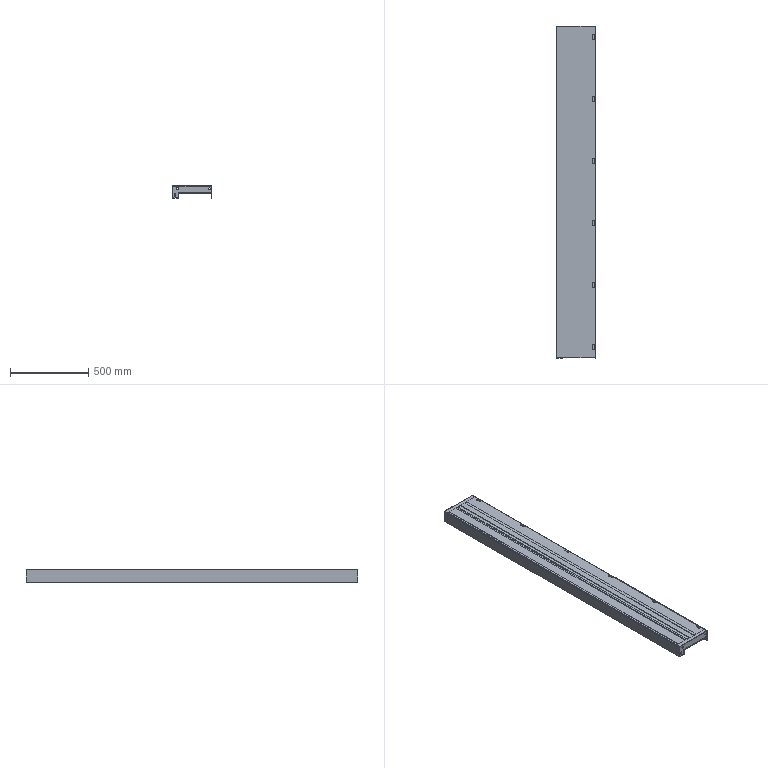Part | SolidWorks | 8 solids | 566 faces | box 251 x 2116 x 80 mm | volume 2427688 mm3 | plane 332 | cylinder 234 | commonest cylinder face diameters 6 x116 6.2 x28 9 x18 2 x11 6.1 x10 11 x10